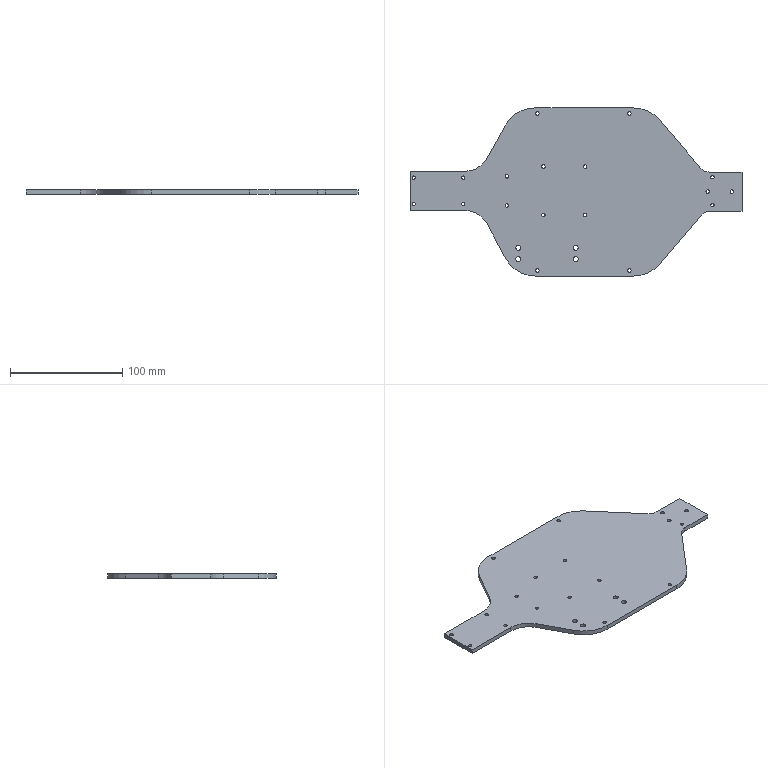Part | STEP file | Wytnij-wyci_gni_cie1_5 | 1 solid | 44 faces | box 296.104 x 150 x 4 mm | volume 113905 mm3 | cylinder 30 | plane 14 | commonest cylinder face diameters 3.1 x6 3 x4 3.16 x4 3.2 x4 4.4 x4 60 x4